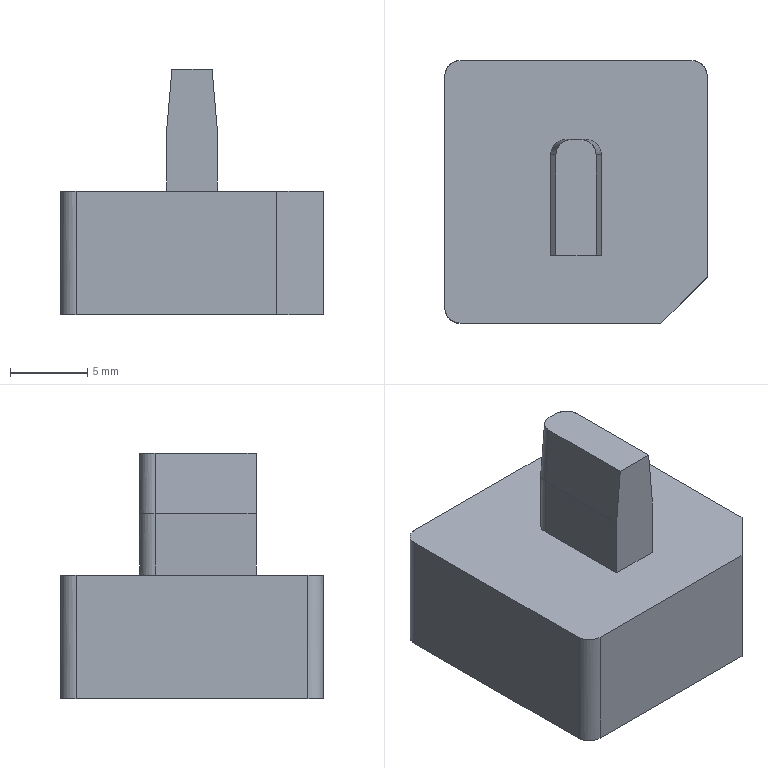NC program | PowerMill | posted with a generic post | part box 17 x 17 x 15.883 mm
Lines 22765 to 22972 of 22972:
N22862 M6
N22863 S15000 M03
N22864 G00 G90 X0.0 Y0.0
N22865 G43 Z10.304 H13
N22866
N22867 G05 P10000 R8
N22868 X-5.9734 Y-7.7954
N22869 Z-8.03
N22870 G01 Z-8.13
N22871 X-6.1351 Y-7.755 F1000.0
N22872 X-6.2541 Y-7.6675
N22873 X-6.3272 Y-7.5378
N22874 X-6.3516 Y-7.3705
N22875 X-6.3282 Y-7.213
N22876 X-6.258 Y-7.0849
N22877 X-6.1404 Y-6.9938
N22878 X-5.9884 Y-6.9635
N22879 X-5.9008 Y-6.9769
N22880 X-5.8112 Y-7.0172
N22881 X-5.6918 Y-7.1307
N22882 X-5.6572 Y-7.1884
N22883 X-5.5281 Y-7.4839
N22884 X-5.4022 Y-7.6442
N22885 X-5.2311 Y-7.7705
N22886 X-5.04 Y-7.8253
N22887 Y-6.9625
N22888 G00 Z-4.8788
N22889 G01 X-5.7197 Y-5.5367 F10000.0
N22890 G00 Z-8.03
N22891 G01 Z-8.13 F600.0
N22892 X-5.6515 Y-5.6113 F1000.0
N22893 X-5.5704 Y-5.7536
N22894 X-5.5047 Y-5.9056
N22895 X-5.4828 Y-6.0093
N22896 X-5.5149 Y-6.1678
N22897 X-5.6112 Y-6.293
N22898 X-5.7463 Y-6.3698
N22899 X-5.9107 Y-6.3955
N22900 X-6.0834 Y-6.3681
N22901 X-6.2232 Y-6.286
N22902 X-6.3195 Y-6.1534
N22903 X-6.3516 Y-5.9845
N22904 X-6.3288 Y-5.8348
N22905 X-6.2605 Y-5.7147
N22906 X-6.1466 Y-5.6242
N22907 X-5.9598 Y-5.5586
N22908 X-5.7197 Y-5.5367
N22909 X-5.4565 Y-5.5588
N22910 X-5.252 Y-5.6252
N22911 X-5.122 Y-5.7191
N22912 X-5.0441 Y-5.8455
N22913 X-5.0181 Y-6.0044
N22914 X-5.0395 Y-6.1436
N22915 X-5.1037 Y-6.2546
N22916 X-5.2059 Y-6.3324
N22917 X-5.3415 Y-6.3716
N22918 G00 Z-4.8788
N22919 G01 X-5.5007 Y-4.5109 F10000.0
N22920 G00 Z-8.03
N22921 G01 Z-8.13 F600.0
N22922 Y-5.0114 F1000.0
N22923 G00 Z-4.8788
N22924 G01 X-5.454 Y-2.8154 F10000.0
N22925 G00 Z-8.03
N22926 G01 Z-8.13 F600.0
N22927 X-5.2711 Y-2.8893 F1000.0
N22928 X-5.1345 Y-3.0054
N22929 X-5.0472 Y-3.1632
N22930 X-5.0181 Y-3.3557
N22931 X-5.039 Y-3.5413
N22932 X-5.1017 Y-3.6941
N22933 X-5.2062 Y-3.814
N22934 X-5.3525 Y-3.9011
N22935 X-5.5211 Y-3.9526
N22936 X-5.7028 Y-3.9697
N22937 X-5.8976 Y-3.951
N22938 X-6.0603 Y-3.8948
N22939 X-6.1907 Y-3.8012
N22940 X-6.2889 Y-3.6702
N22941 X-6.3486 Y-3.5189
N22942 X-6.3685 Y-3.3537
N22943 X-6.344 Y-3.1746
N22944 X-6.2705 Y-3.0253
N22945 X-6.1507 Y-2.9112
N22946 X-5.9874 Y-2.8373
N22947 G00 Z-4.8788
N22948 G01 X-5.9242 Y-2.2562 F10000.0
N22949 G00 Z-8.03
N22950 G01 Z-8.13 F600.0
N22951 X-6.1112 Y-2.2051 F1000.0
N22952 X-6.2448 Y-2.1199
N22953 X-6.3249 Y-2.0006
N22954 X-6.3516 Y-1.8473
N22955 X-6.3249 Y-1.694
N22956 X-6.2448 Y-1.5747
N22957 X-6.1112 Y-1.4895
N22958 X-5.9242 Y-1.4384
N22959 X-5.6839 Y-1.4214
N22960 X-5.4251 Y-1.4424
N22961 X-5.2287 Y-1.5054
N22962 X-5.0947 Y-1.6105
N22963 X-5.0373 Y-1.7164
N22964 X-5.0181 Y-1.8473
N22965 X-5.0447 Y-2.0006
N22966 X-5.1246 Y-2.1199
N22967 X-5.2578 Y-2.2051
N22968 X-5.4442 Y-2.2562
N22969 X-5.6839 Y-2.2732
N22970 X-5.9242 Y-2.2562
N22971 G00 Z-4.8788
N22972 G01 X-6.1764 Y-0.5071 F10000.0
N22973 G00 Z-8.03
N22974 G01 Z-8.13 F600.0
N22975 X-6.3456 Y-0.2613 F1000.0
N22976 X-5.04
N22977 G00 Z-4.8788
N22978 G01 X-5.5007 Y1.0203 F10000.0
N22979 G00 Z-8.03
N22980 G01 Z-8.13 F600.0
N22981 Y0.5197 F1000.0
N22982 G00 Z-4.8788
N22983 G01 X-5.3774 Y1.5465 F10000.0
N22984 G00 Z-8.03
N22985 G01 Z-8.13 F600.0
N22986 X-5.2234 Y1.591 F1000.0
N22987 X-5.1097 Y1.6808
N22988 X-5.0417 Y1.8075
N22989 X-5.0191 Y1.9684
N22990 X-5.0549 Y2.1421
N22991 X-5.1624 Y2.2889
N22992 X-5.3114 Y2.3846
N22993 X-5.4818 Y2.4132
N22994 X-5.6474 Y2.3859
N22995 X-5.7669 Y2.3147
N22996 X-5.8405 Y2.1998
N22997 X-5.868 Y2.0411
N22998 X-5.852 Y1.9338
N22999 X-5.8003 Y1.8072
N23000 X-5.7284 Y1.6875
N23001 X-5.644 Y1.5873
N23002 X-6.3287 Y1.6997
N23003 Y2.3456
N23004 G00 Z-4.8788
N23005 G01 X-5.5007 Y3.4311 F10000.0
N23006 G00 Z-8.03
N23007 G01 Z-8.13 F600.0
N23008 Y2.9305 F1000.0
N23009 G00 Z-4.8788
N23010 G01 X-5.5743 Y3.9651 F10000.0
N23011 G00 Z-8.03
N23012 G01 Z-8.13 F600.0
N23013 X-5.6839 Y3.9573 F1000.0
N23014 X-5.9242 Y3.9743
N23015 X-6.1112 Y4.0254
N23016 X-6.2448 Y4.1106
N23017 X-6.3249 Y4.2299
N23018 X-6.3516 Y4.3832
N23019 X-6.3249 Y4.5365
N23020 X-6.2448 Y4.6558
N23021 X-6.1112 Y4.741
N23022 X-5.9242 Y4.7921
N23023 X-5.6839 Y4.8091
N23024 X-5.4251 Y4.7881
N23025 X-5.2287 Y4.7251
N23026 X-5.0947 Y4.62
N23027 X-5.0373 Y4.5141
N23028 X-5.0181 Y4.3832
N23029 X-5.0447 Y4.2299
N23030 X-5.1246 Y4.1106
N23031 X-5.2578 Y4.0254
N23032 X-5.4442 Y3.9743
N23033 X-5.5743 Y3.9651
N23034 G00 Z-4.8788
N23035 G01 X-5.1057 Y5.5364 F10000.0
N23036 G00 Z-8.03
N23037 G01 Z-8.13 F600.0
N23038 X-5.2864 F1000.0
N23039 G00 Z-4.8788
N23040 G01 X-5.9734 Y6.2765 F10000.0
N23041 G00 Z-8.03
N23042 G01 Z-8.13 F600.0
N23043 X-6.1351 Y6.317 F1000.0
N23044 X-6.2541 Y6.4044
N23045 X-6.3272 Y6.5342
N23046 X-6.3516 Y6.7015
N23047 X-6.3282 Y6.8589
N23048 X-6.258 Y6.9871
N23049 X-6.1404 Y7.0781
N23050 X-5.9884 Y7.1085
N23051 X-5.9008 Y7.095
N23052 X-5.8112 Y7.0547
N23053 X-5.6918 Y6.9413
N23054 X-5.6572 Y6.8836
N23055 X-5.5281 Y6.588
N23056 X-5.4022 Y6.4278
N23057 X-5.2311 Y6.3014
N23058 X-5.04 Y6.2467
N23059 Y7.1095
N23060 G00 Z10.304
N23061 G05 P0
N23062 (---------------)
N23063 ( END TOOLPATH : 粗公刻字01-刻字-TEXT_D4 )
N23064 (---------------)
N23065
N23066 M05
N23067 G53 Z0.0
N23068 M30
%